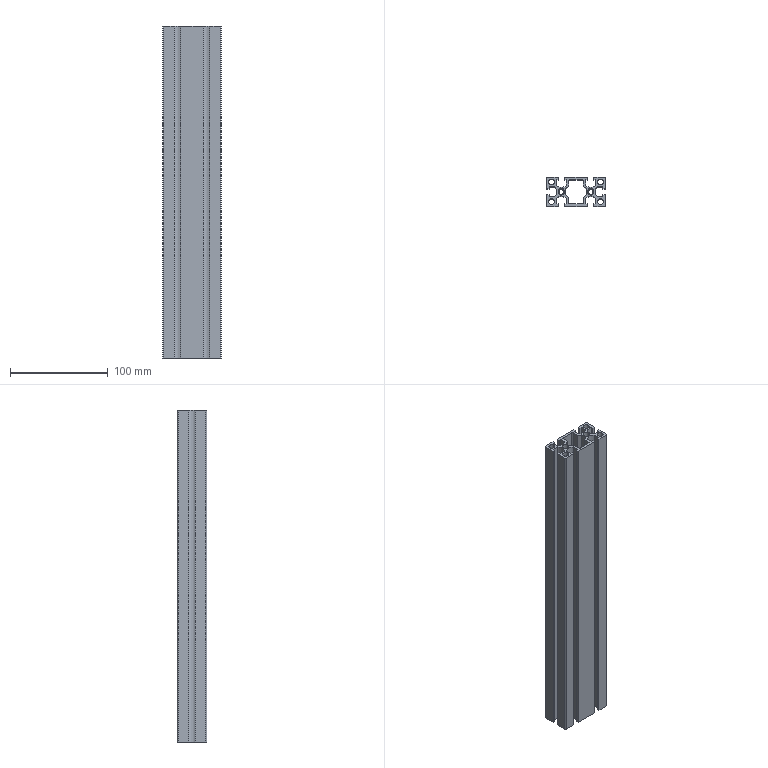Part | STEP file | 08-14 equal-height profile | 1 solid | 103 faces | box 60 x 30 x 340 mm | volume 224122 mm3 | plane 60 | cylinder 35 | cone 8 | commonest cylinder face diameters 2 x8 6 x8 6.8 x8 15 x7 5 x4